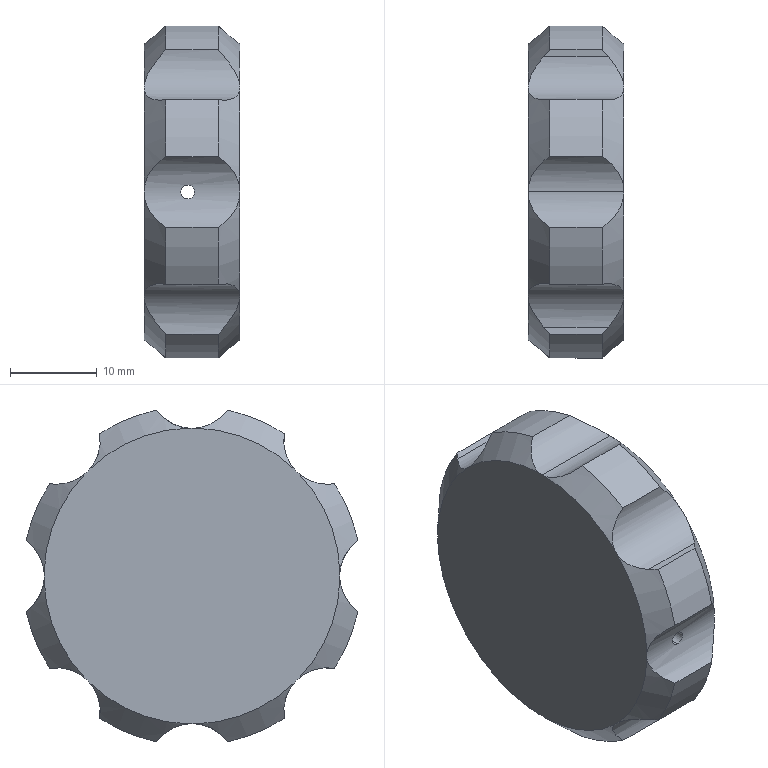Part | SolidWorks | features BaseBody 1 | 1 solid | 47 faces | box 11 x 38.188 x 38.188 mm | volume 8381 mm3 | cylinder 27 | cone 16 | plane 4 | commonest cylinder face diameters 10 x11 39.045 x8 1.6 x4 22 x2 24 x2